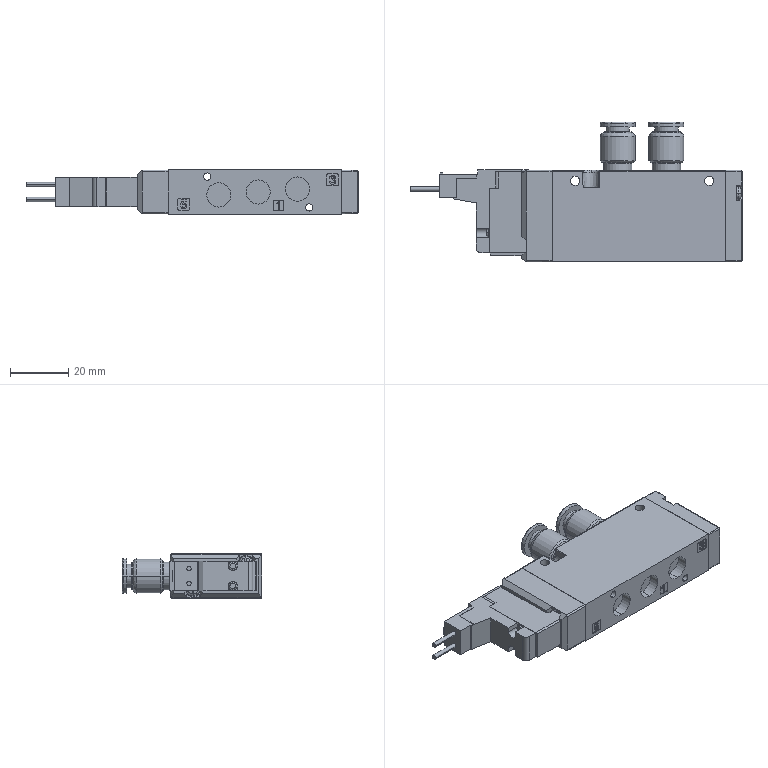Part | STEP file | 4RD219-GS6-E2-3_default | 13 solids | 692 faces | box 113.84 x 47.8 x 15.298 mm | volume 40931 mm3 | plane 318 | cylinder 223 | spline 94 | cone 57 | commonest cylinder face diameters 0.6 x44 2.5 x20 8.3 x10 1 x8 2.208 x8 2.6 x8